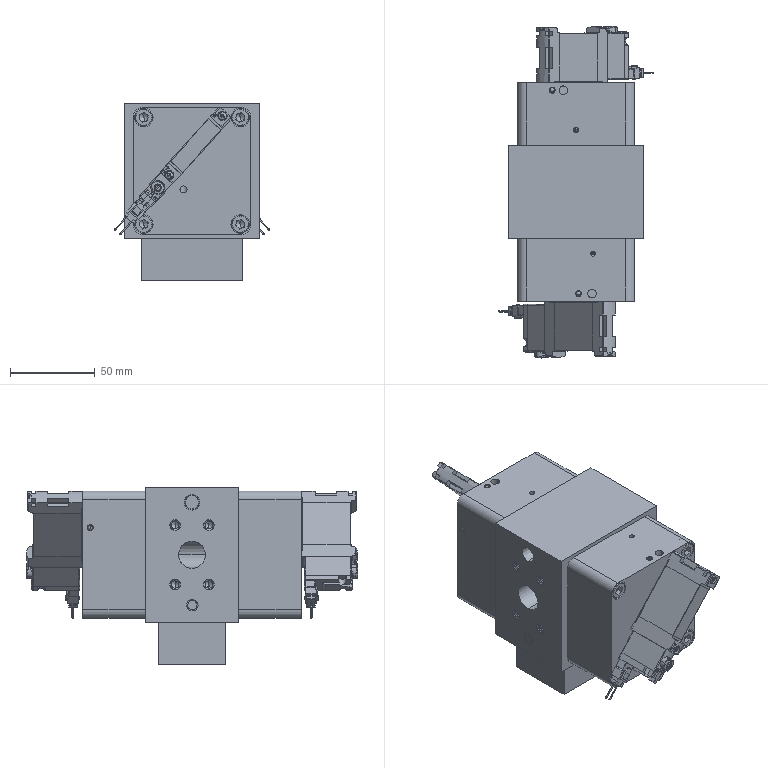Part | STEP file | PN_0049_default | 59 solids | 2645 faces | box 91.232 x 195.93 x 105 mm | volume 684880 mm3 | plane 1302 | cylinder 743 | cone 254 | torus 214 | spline 114 | sphere 18 | commonest cylinder face diameters 3 x64 1 x56 0.4 x36 6.3 x36 10 x35 5 x29